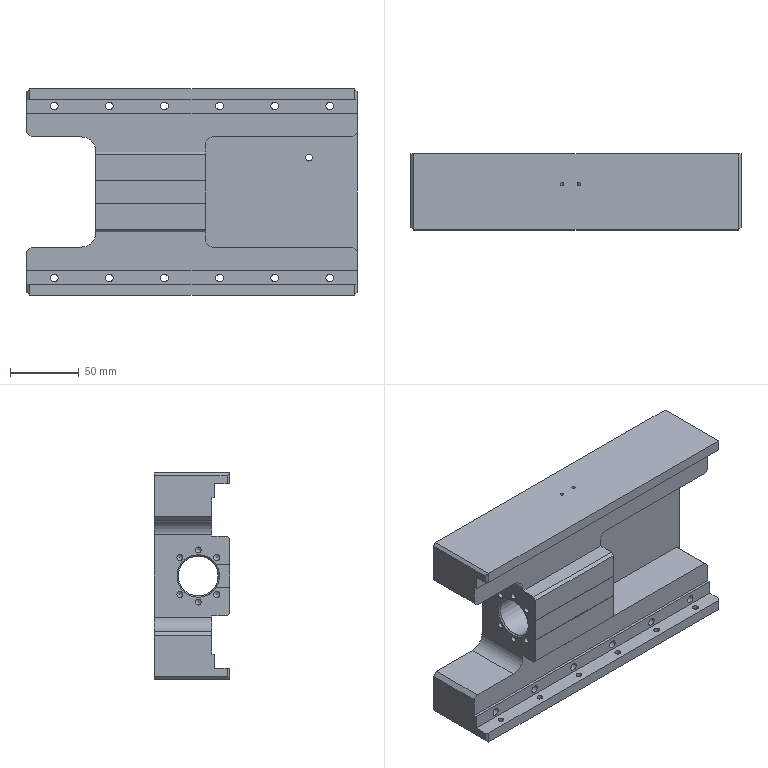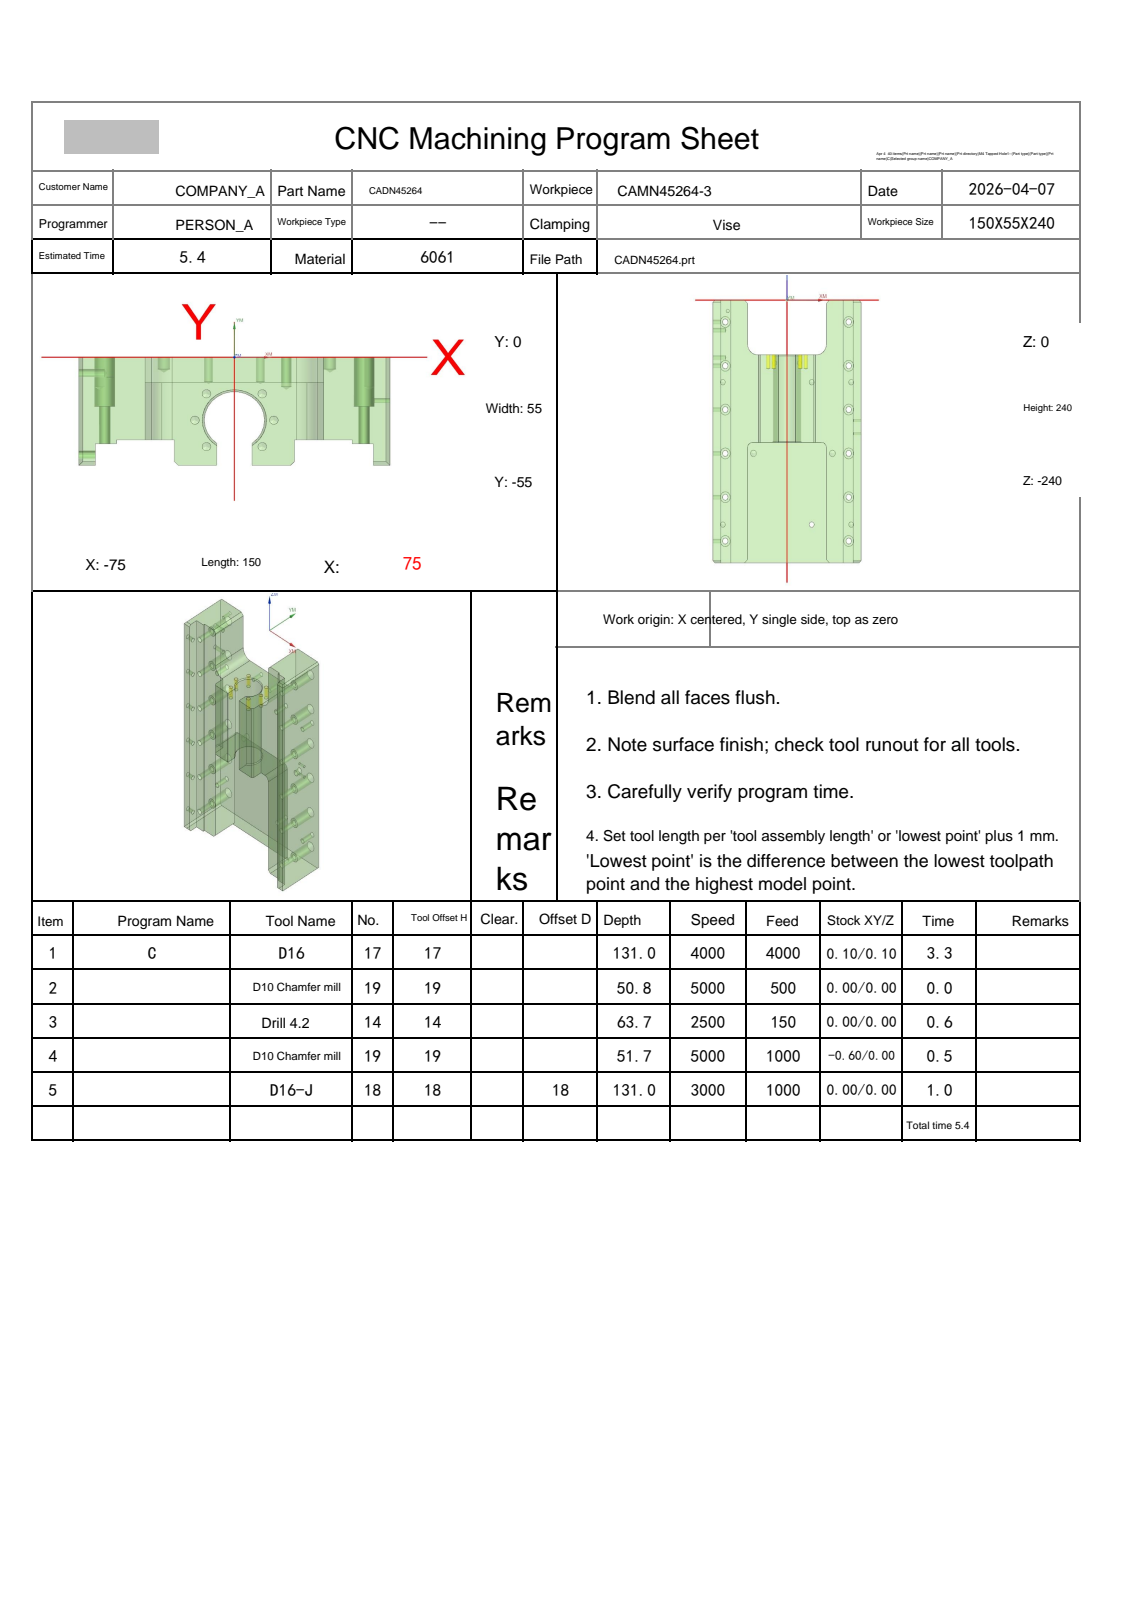NC program | NX | posted by the shop | part box 240 x 55 x 150 mm
Whole program, first 1628 of 1926 lines:
%
O0001
(Machine time: 6.41 MIN)
(===Total Tool:4===)
(T17=D16    D=16.  R=0.   D-  H17 Z=-131. )
(T19=D10 Chamfer mill D=10.  R=0.   D-  H19 Z=-51.7 )
(T14=Drill 4.2  D=4.2  DR_a=118 D-  H14 Z=-63.66)
(T18=D16-J  D=16.  R=0.   D18 H18 Z=-131. )
G80 G90 G17 G49 G40
G91 G28 Z0
M01
N1 T17 M06
(D16  D=16. R=0. H=17 ce=0.10 di=0.10)
G00 G90 G54 X.4 Y-68.796 M03 S4000
G43 H17 Z20.
M08
Z-50.6
G01 Y-54.8 F4000.
Y-44.285
G02 X3.874 Y-37.538 I8.289 J-.001
G03 X6.759 Y-32. I-3.874 J5.538
X0.0 Y-25.241 I-6.759 J0.0
X-6.759 Y-32. I0.0 J-6.759
X-3.908 Y-37.514 I6.759 J0.0
G02 X-.4 Y-44.285 I-4.781 J-6.771
G01 Y-54.8
Y-68.796
G00 Z-51.2
G01 Y-54.8
Y-43.747
G03 X-3.752 Y-37.185 I-8.1 J0.0
G02 X-6.4 Y-32. I3.752 J5.185
X0.0 Y-25.6 I6.4 J0.0
X6.4 Y-32. I0.0 J-6.4
X3.752 Y-37.185 I-6.4 J0.0
G03 X.4 Y-43.747 I4.748 J-6.562
G01 Y-54.8
Y-68.796
G00 Z-51.8
G01 Y-54.8
Y-43.747
G02 X3.752 Y-37.185 I8.1 J0.0
G03 X6.4 Y-32. I-3.752 J5.185
X0.0 Y-25.6 I-6.4 J0.0
X-6.4 Y-32. I0.0 J-6.4
X-3.752 Y-37.185 I6.4 J0.0
G02 X-.4 Y-43.747 I-4.748 J-6.562
G01 Y-54.8
Y-68.796
G00 Z-52.4
G01 Y-54.8
Y-43.747
G03 X-3.752 Y-37.185 I-8.1 J0.0
G02 X-6.4 Y-32. I3.752 J5.185
X0.0 Y-25.6 I6.4 J0.0
X6.4 Y-32. I0.0 J-6.4
X3.752 Y-37.185 I-6.4 J0.0
G03 X.4 Y-43.747 I4.748 J-6.562
G01 Y-54.8
Y-68.796
G00 Z-53.
G01 Y-54.8
Y-43.747
G02 X3.752 Y-37.185 I8.1 J0.0
G03 X6.4 Y-32. I-3.752 J5.185
X0.0 Y-25.6 I-6.4 J0.0
X-6.4 Y-32. I0.0 J-6.4
X-3.752 Y-37.185 I6.4 J0.0
G02 X-.4 Y-43.747 I-4.748 J-6.562
G01 Y-54.8
Y-68.796
G00 Z-53.6
G01 Y-54.8
Y-43.747
G03 X-3.752 Y-37.185 I-8.1 J0.0
G02 X-6.4 Y-32. I3.752 J5.185
X0.0 Y-25.6 I6.4 J0.0
X6.4 Y-32. I0.0 J-6.4
X3.752 Y-37.185 I-6.4 J0.0
G03 X.4 Y-43.747 I4.748 J-6.562
G01 Y-54.8
Y-68.796
G00 Z-54.2
G01 Y-54.8
Y-43.747
G02 X3.752 Y-37.185 I8.1 J0.0
G03 X6.4 Y-32. I-3.752 J5.185
X0.0 Y-25.6 I-6.4 J0.0
X-6.4 Y-32. I0.0 J-6.4
X-3.752 Y-37.185 I6.4 J0.0
G02 X-.4 Y-43.747 I-4.748 J-6.562
G01 Y-54.8
Y-68.796
G00 Z-54.8
G01 Y-54.8
Y-43.747
G03 X-3.752 Y-37.185 I-8.1 J0.0
G02 X-6.4 Y-32. I3.752 J5.185
X0.0 Y-25.6 I6.4 J0.0
X6.4 Y-32. I0.0 J-6.4
X3.752 Y-37.185 I-6.4 J0.0
G03 X.4 Y-43.747 I4.748 J-6.562
G01 Y-54.8
Y-68.796
G00 Z-55.4
G01 Y-54.8
Y-43.747
G02 X3.752 Y-37.185 I8.1 J0.0
G03 X6.4 Y-32. I-3.752 J5.185
X0.0 Y-25.6 I-6.4 J0.0
X-6.4 Y-32. I0.0 J-6.4
X-3.752 Y-37.185 I6.4 J0.0
G02 X-.4 Y-43.747 I-4.748 J-6.562
G01 Y-54.8
Y-68.796
G00 Z-56.
G01 Y-54.8
Y-43.747
G03 X-3.752 Y-37.185 I-8.1 J0.0
G02 X-6.4 Y-32. I3.752 J5.185
X0.0 Y-25.6 I6.4 J0.0
X6.4 Y-32. I0.0 J-6.4
X3.752 Y-37.185 I-6.4 J0.0
G03 X.4 Y-43.747 I4.748 J-6.562
G01 Y-54.8
Y-68.796
G00 Z-56.6
G01 Y-54.8
Y-43.747
G02 X3.752 Y-37.185 I8.1 J0.0
G03 X6.4 Y-32. I-3.752 J5.185
X0.0 Y-25.6 I-6.4 J0.0
X-6.4 Y-32. I0.0 J-6.4
X-3.752 Y-37.185 I6.4 J0.0
G02 X-.4 Y-43.747 I-4.748 J-6.562
G01 Y-54.8
Y-68.796
G00 Z-57.2
G01 Y-54.8
Y-43.747
G03 X-3.752 Y-37.185 I-8.1 J0.0
G02 X-6.4 Y-32. I3.752 J5.185
X0.0 Y-25.6 I6.4 J0.0
X6.4 Y-32. I0.0 J-6.4
X3.752 Y-37.185 I-6.4 J0.0
G03 X.4 Y-43.747 I4.748 J-6.562
G01 Y-54.8
Y-68.796
G00 Z-57.8
G01 Y-54.8
Y-43.747
G02 X3.752 Y-37.185 I8.1 J0.0
G03 X6.4 Y-32. I-3.752 J5.185
X0.0 Y-25.6 I-6.4 J0.0
X-6.4 Y-32. I0.0 J-6.4
X-3.752 Y-37.185 I6.4 J0.0
G02 X-.4 Y-43.747 I-4.748 J-6.562
G01 Y-54.8
Y-68.796
G00 Z-58.4
G01 Y-54.8
Y-43.747
G03 X-3.752 Y-37.185 I-8.1 J0.0
G02 X-6.4 Y-32. I3.752 J5.185
X0.0 Y-25.6 I6.4 J0.0
X6.4 Y-32. I0.0 J-6.4
X3.752 Y-37.185 I-6.4 J0.0
G03 X.4 Y-43.747 I4.748 J-6.562
G01 Y-54.8
Y-68.796
G00 Z-59.
G01 Y-54.8
Y-43.747
G02 X3.752 Y-37.185 I8.1 J0.0
G03 X6.4 Y-32. I-3.752 J5.185
X0.0 Y-25.6 I-6.4 J0.0
X-6.4 Y-32. I0.0 J-6.4
X-3.752 Y-37.185 I6.4 J0.0
G02 X-.4 Y-43.747 I-4.748 J-6.562
G01 Y-54.8
Y-68.796
G00 Z-59.6
G01 Y-54.8
Y-43.747
G03 X-3.752 Y-37.185 I-8.1 J0.0
G02 X-6.4 Y-32. I3.752 J5.185
X0.0 Y-25.6 I6.4 J0.0
X6.4 Y-32. I0.0 J-6.4
X3.752 Y-37.185 I-6.4 J0.0
G03 X.4 Y-43.747 I4.748 J-6.562
G01 Y-54.8
Y-68.796
G00 Z-60.2
G01 Y-54.8
Y-43.747
G02 X3.752 Y-37.185 I8.1 J0.0
G03 X6.4 Y-32. I-3.752 J5.185
X0.0 Y-25.6 I-6.4 J0.0
X-6.4 Y-32. I0.0 J-6.4
X-3.752 Y-37.185 I6.4 J0.0
G02 X-.4 Y-43.747 I-4.748 J-6.562
G01 Y-54.8
Y-68.796
G00 Z-60.8
G01 Y-54.8
Y-43.747
G03 X-3.752 Y-37.185 I-8.1 J0.0
G02 X-6.4 Y-32. I3.752 J5.185
X0.0 Y-25.6 I6.4 J0.0
X6.4 Y-32. I0.0 J-6.4
X3.752 Y-37.185 I-6.4 J0.0
G03 X.4 Y-43.747 I4.748 J-6.562
G01 Y-54.8
Y-68.796
G00 Z-61.4
G01 Y-54.8
Y-43.747
G02 X3.752 Y-37.185 I8.1 J0.0
G03 X6.4 Y-32. I-3.752 J5.185
X0.0 Y-25.6 I-6.4 J0.0
X-6.4 Y-32. I0.0 J-6.4
X-3.752 Y-37.185 I6.4 J0.0
G02 X-.4 Y-43.747 I-4.748 J-6.562
G01 Y-54.8
Y-68.796
G00 Z-62.
G01 Y-54.8
Y-43.747
G03 X-3.752 Y-37.185 I-8.1 J0.0
G02 X-6.4 Y-32. I3.752 J5.185
X0.0 Y-25.6 I6.4 J0.0
X6.4 Y-32. I0.0 J-6.4
X3.752 Y-37.185 I-6.4 J0.0
G03 X.4 Y-43.747 I4.748 J-6.562
G01 Y-54.8
Y-68.796
G00 Z-62.6
G01 Y-54.8
Y-43.747
G02 X3.752 Y-37.185 I8.1 J0.0
G03 X6.4 Y-32. I-3.752 J5.185
X0.0 Y-25.6 I-6.4 J0.0
X-6.4 Y-32. I0.0 J-6.4
X-3.752 Y-37.185 I6.4 J0.0
G02 X-.4 Y-43.747 I-4.748 J-6.562
G01 Y-54.8
Y-68.796
G00 Z-63.2
G01 Y-54.8
Y-43.747
G03 X-3.752 Y-37.185 I-8.1 J0.0
G02 X-6.4 Y-32. I3.752 J5.185
X0.0 Y-25.6 I6.4 J0.0
X6.4 Y-32. I0.0 J-6.4
X3.752 Y-37.185 I-6.4 J0.0
G03 X.4 Y-43.747 I4.748 J-6.562
G01 Y-54.8
Y-68.796
G00 Z-63.8
G01 Y-54.8
Y-43.747
G02 X3.752 Y-37.185 I8.1 J0.0
G03 X6.4 Y-32. I-3.752 J5.185
X0.0 Y-25.6 I-6.4 J0.0
X-6.4 Y-32. I0.0 J-6.4
X-3.752 Y-37.185 I6.4 J0.0
G02 X-.4 Y-43.747 I-4.748 J-6.562
G01 Y-54.8
Y-68.796
G00 Z-64.4
G01 Y-54.8
Y-43.747
G03 X-3.752 Y-37.185 I-8.1 J0.0
G02 X-6.4 Y-32. I3.752 J5.185
X0.0 Y-25.6 I6.4 J0.0
X6.4 Y-32. I0.0 J-6.4
X3.752 Y-37.185 I-6.4 J0.0
G03 X.4 Y-43.747 I4.748 J-6.562
G01 Y-54.8
Y-68.796
G00 Z-65.
G01 Y-54.8
Y-43.747
G02 X3.752 Y-37.185 I8.1 J0.0
G03 X6.4 Y-32. I-3.752 J5.185
X0.0 Y-25.6 I-6.4 J0.0
X-6.4 Y-32. I0.0 J-6.4
X-3.752 Y-37.185 I6.4 J0.0
G02 X-.4 Y-43.747 I-4.748 J-6.562
G01 Y-54.8
Y-68.796
G00 Z-65.6
G01 Y-54.8
Y-43.747
G03 X-3.752 Y-37.185 I-8.1 J0.0
G02 X-6.4 Y-32. I3.752 J5.185
X0.0 Y-25.6 I6.4 J0.0
X6.4 Y-32. I0.0 J-6.4
X3.752 Y-37.185 I-6.4 J0.0
G03 X.4 Y-43.747 I4.748 J-6.562
G01 Y-54.8
Y-68.796
G00 Z-66.2
G01 Y-54.8
Y-43.747
G02 X3.752 Y-37.185 I8.1 J0.0
G03 X6.4 Y-32. I-3.752 J5.185
X0.0 Y-25.6 I-6.4 J0.0
X-6.4 Y-32. I0.0 J-6.4
X-3.752 Y-37.185 I6.4 J0.0
G02 X-.4 Y-43.747 I-4.748 J-6.562
G01 Y-54.8
Y-68.796
G00 Z-66.8
G01 Y-54.8
Y-43.747
G03 X-3.752 Y-37.185 I-8.1 J0.0
G02 X-6.4 Y-32. I3.752 J5.185
X0.0 Y-25.6 I6.4 J0.0
X6.4 Y-32. I0.0 J-6.4
X3.752 Y-37.185 I-6.4 J0.0
G03 X.4 Y-43.747 I4.748 J-6.562
G01 Y-54.8
Y-68.796
G00 Z-67.4
G01 Y-54.8
Y-43.747
G02 X3.752 Y-37.185 I8.1 J0.0
G03 X6.4 Y-32. I-3.752 J5.185
X0.0 Y-25.6 I-6.4 J0.0
X-6.4 Y-32. I0.0 J-6.4
X-3.752 Y-37.185 I6.4 J0.0
G02 X-.4 Y-43.747 I-4.748 J-6.562
G01 Y-54.8
Y-68.796
G00 Z-68.
G01 Y-54.8
Y-43.747
G03 X-3.752 Y-37.185 I-8.1 J0.0
G02 X-6.4 Y-32. I3.752 J5.185
X0.0 Y-25.6 I6.4 J0.0
X6.4 Y-32. I0.0 J-6.4
X3.752 Y-37.185 I-6.4 J0.0
G03 X.4 Y-43.747 I4.748 J-6.562
G01 Y-54.8
Y-68.796
G00 Z-68.6
G01 Y-54.8
Y-43.747
G02 X3.752 Y-37.185 I8.1 J0.0
G03 X6.4 Y-32. I-3.752 J5.185
X0.0 Y-25.6 I-6.4 J0.0
X-6.4 Y-32. I0.0 J-6.4
X-3.752 Y-37.185 I6.4 J0.0
G02 X-.4 Y-43.747 I-4.748 J-6.562
G01 Y-54.8
Y-68.796
G00 Z-69.2
G01 Y-54.8
Y-43.747
G03 X-3.752 Y-37.185 I-8.1 J0.0
G02 X-6.4 Y-32. I3.752 J5.185
X0.0 Y-25.6 I6.4 J0.0
X6.4 Y-32. I0.0 J-6.4
X3.752 Y-37.185 I-6.4 J0.0
G03 X.4 Y-43.747 I4.748 J-6.562
G01 Y-54.8
Y-68.796
G00 Z-69.8
G01 Y-54.8
Y-43.747
G02 X3.752 Y-37.185 I8.1 J0.0
G03 X6.4 Y-32. I-3.752 J5.185
X0.0 Y-25.6 I-6.4 J0.0
X-6.4 Y-32. I0.0 J-6.4
X-3.752 Y-37.185 I6.4 J0.0
G02 X-.4 Y-43.747 I-4.748 J-6.562
G01 Y-54.8
Y-68.796
G00 Z-70.4
G01 Y-54.8
Y-43.747
G03 X-3.752 Y-37.185 I-8.1 J0.0
G02 X-6.4 Y-32. I3.752 J5.185
X0.0 Y-25.6 I6.4 J0.0
X6.4 Y-32. I0.0 J-6.4
X3.752 Y-37.185 I-6.4 J0.0
G03 X.4 Y-43.747 I4.748 J-6.562
G01 Y-54.8
Y-68.796
G00 Z-71.
G01 Y-54.8
Y-43.747
G02 X3.752 Y-37.185 I8.1 J0.0
G03 X6.4 Y-32. I-3.752 J5.185
X0.0 Y-25.6 I-6.4 J0.0
X-6.4 Y-32. I0.0 J-6.4
X-3.752 Y-37.185 I6.4 J0.0
G02 X-.4 Y-43.747 I-4.748 J-6.562
G01 Y-54.8
Y-68.796
G00 Z-71.6
G01 Y-54.8
Y-43.747
G03 X-3.752 Y-37.185 I-8.1 J0.0
G02 X-6.4 Y-32. I3.752 J5.185
X0.0 Y-25.6 I6.4 J0.0
X6.4 Y-32. I0.0 J-6.4
X3.752 Y-37.185 I-6.4 J0.0
G03 X.4 Y-43.747 I4.748 J-6.562
G01 Y-54.8
Y-68.796
G00 Z-72.2
G01 Y-54.8
Y-43.747
G02 X3.752 Y-37.185 I8.1 J0.0
G03 X6.4 Y-32. I-3.752 J5.185
X0.0 Y-25.6 I-6.4 J0.0
X-6.4 Y-32. I0.0 J-6.4
X-3.752 Y-37.185 I6.4 J0.0
G02 X-.4 Y-43.747 I-4.748 J-6.562
G01 Y-54.8
Y-68.796
G00 Z-72.8
G01 Y-54.8
Y-43.747
G03 X-3.752 Y-37.185 I-8.1 J0.0
G02 X-6.4 Y-32. I3.752 J5.185
X0.0 Y-25.6 I6.4 J0.0
X6.4 Y-32. I0.0 J-6.4
X3.752 Y-37.185 I-6.4 J0.0
G03 X.4 Y-43.747 I4.748 J-6.562
G01 Y-54.8
Y-68.796
G00 Z-73.4
G01 Y-54.8
Y-43.747
G02 X3.752 Y-37.185 I8.1 J0.0
G03 X6.4 Y-32. I-3.752 J5.185
X0.0 Y-25.6 I-6.4 J0.0
X-6.4 Y-32. I0.0 J-6.4
X-3.752 Y-37.185 I6.4 J0.0
G02 X-.4 Y-43.747 I-4.748 J-6.562
G01 Y-54.8
Y-68.796
G00 Z-74.
G01 Y-54.8
Y-43.747
G03 X-3.752 Y-37.185 I-8.1 J0.0
G02 X-6.4 Y-32. I3.752 J5.185
X0.0 Y-25.6 I6.4 J0.0
X6.4 Y-32. I0.0 J-6.4
X3.752 Y-37.185 I-6.4 J0.0
G03 X.4 Y-43.747 I4.748 J-6.562
G01 Y-54.8
Y-68.796
G00 Z-74.6
G01 Y-54.8
Y-43.747
G02 X3.752 Y-37.185 I8.1 J0.0
G03 X6.4 Y-32. I-3.752 J5.185
X0.0 Y-25.6 I-6.4 J0.0
X-6.4 Y-32. I0.0 J-6.4
X-3.752 Y-37.185 I6.4 J0.0
G02 X-.4 Y-43.747 I-4.748 J-6.562
G01 Y-54.8
Y-68.796
G00 Z-75.2
G01 Y-54.8
Y-43.747
G03 X-3.752 Y-37.185 I-8.1 J0.0
G02 X-6.4 Y-32. I3.752 J5.185
X0.0 Y-25.6 I6.4 J0.0
X6.4 Y-32. I0.0 J-6.4
X3.752 Y-37.185 I-6.4 J0.0
G03 X.4 Y-43.747 I4.748 J-6.562
G01 Y-54.8
Y-68.796
G00 Z-75.8
G01 Y-54.8
Y-43.747
G02 X3.752 Y-37.185 I8.1 J0.0
G03 X6.4 Y-32. I-3.752 J5.185
X0.0 Y-25.6 I-6.4 J0.0
X-6.4 Y-32. I0.0 J-6.4
X-3.752 Y-37.185 I6.4 J0.0
G02 X-.4 Y-43.747 I-4.748 J-6.562
G01 Y-54.8
Y-68.796
G00 Z-76.4
G01 Y-54.8
Y-43.747
G03 X-3.752 Y-37.185 I-8.1 J0.0
G02 X-6.4 Y-32. I3.752 J5.185
X0.0 Y-25.6 I6.4 J0.0
X6.4 Y-32. I0.0 J-6.4
X3.752 Y-37.185 I-6.4 J0.0
G03 X.4 Y-43.747 I4.748 J-6.562
G01 Y-54.8
Y-68.796
G00 Z-77.
G01 Y-54.8
Y-43.747
G02 X3.752 Y-37.185 I8.1 J0.0
G03 X6.4 Y-32. I-3.752 J5.185
X0.0 Y-25.6 I-6.4 J0.0
X-6.4 Y-32. I0.0 J-6.4
X-3.752 Y-37.185 I6.4 J0.0
G02 X-.4 Y-43.747 I-4.748 J-6.562
G01 Y-54.8
Y-68.796
G00 Z-77.6
G01 Y-54.8
Y-43.747
G03 X-3.752 Y-37.185 I-8.1 J0.0
G02 X-6.4 Y-32. I3.752 J5.185
X0.0 Y-25.6 I6.4 J0.0
X6.4 Y-32. I0.0 J-6.4
X3.752 Y-37.185 I-6.4 J0.0
G03 X.4 Y-43.747 I4.748 J-6.562
G01 Y-54.8
Y-68.796
G00 Z-78.2
G01 Y-54.8
Y-43.747
G02 X3.752 Y-37.185 I8.1 J0.0
G03 X6.4 Y-32. I-3.752 J5.185
X0.0 Y-25.6 I-6.4 J0.0
X-6.4 Y-32. I0.0 J-6.4
X-3.752 Y-37.185 I6.4 J0.0
G02 X-.4 Y-43.747 I-4.748 J-6.562
G01 Y-54.8
Y-68.796
G00 Z-78.8
G01 Y-54.8
Y-43.747
G03 X-3.752 Y-37.185 I-8.1 J0.0
G02 X-6.4 Y-32. I3.752 J5.185
X0.0 Y-25.6 I6.4 J0.0
X6.4 Y-32. I0.0 J-6.4
X3.752 Y-37.185 I-6.4 J0.0
G03 X.4 Y-43.747 I4.748 J-6.562
G01 Y-54.8
Y-68.796
G00 Z-79.4
G01 Y-54.8
Y-43.747
G02 X3.752 Y-37.185 I8.1 J0.0
G03 X6.4 Y-32. I-3.752 J5.185
X0.0 Y-25.6 I-6.4 J0.0
X-6.4 Y-32. I0.0 J-6.4
X-3.752 Y-37.185 I6.4 J0.0
G02 X-.4 Y-43.747 I-4.748 J-6.562
G01 Y-54.8
Y-68.796
G00 Z-80.
G01 Y-54.8
Y-43.747
G03 X-3.752 Y-37.185 I-8.1 J0.0
G02 X-6.4 Y-32. I3.752 J5.185
X0.0 Y-25.6 I6.4 J0.0
X6.4 Y-32. I0.0 J-6.4
X3.752 Y-37.185 I-6.4 J0.0
G03 X.4 Y-43.747 I4.748 J-6.562
G01 Y-54.8
Y-68.796
G00 Z-80.6
G01 Y-54.8
Y-43.747
G02 X3.752 Y-37.185 I8.1 J0.0
G03 X6.4 Y-32. I-3.752 J5.185
X0.0 Y-25.6 I-6.4 J0.0
X-6.4 Y-32. I0.0 J-6.4
X-3.752 Y-37.185 I6.4 J0.0
G02 X-.4 Y-43.747 I-4.748 J-6.562
G01 Y-54.8
Y-68.796
G00 Z-81.2
G01 Y-54.8
Y-43.747
G03 X-3.752 Y-37.185 I-8.1 J0.0
G02 X-6.4 Y-32. I3.752 J5.185
X0.0 Y-25.6 I6.4 J0.0
X6.4 Y-32. I0.0 J-6.4
X3.752 Y-37.185 I-6.4 J0.0
G03 X.4 Y-43.747 I4.748 J-6.562
G01 Y-54.8
Y-68.796
G00 Z-81.8
G01 Y-54.8
Y-43.747
G02 X3.752 Y-37.185 I8.1 J0.0
G03 X6.4 Y-32. I-3.752 J5.185
X0.0 Y-25.6 I-6.4 J0.0
X-6.4 Y-32. I0.0 J-6.4
X-3.752 Y-37.185 I6.4 J0.0
G02 X-.4 Y-43.747 I-4.748 J-6.562
G01 Y-54.8
Y-68.796
G00 Z-82.4
G01 Y-54.8
Y-43.747
G03 X-3.752 Y-37.185 I-8.1 J0.0
G02 X-6.4 Y-32. I3.752 J5.185
X0.0 Y-25.6 I6.4 J0.0
X6.4 Y-32. I0.0 J-6.4
X3.752 Y-37.185 I-6.4 J0.0
G03 X.4 Y-43.747 I4.748 J-6.562
G01 Y-54.8
Y-68.796
G00 Z-83.
G01 Y-54.8
Y-43.747
G02 X3.752 Y-37.185 I8.1 J0.0
G03 X6.4 Y-32. I-3.752 J5.185
X0.0 Y-25.6 I-6.4 J0.0
X-6.4 Y-32. I0.0 J-6.4
X-3.752 Y-37.185 I6.4 J0.0
G02 X-.4 Y-43.747 I-4.748 J-6.562
G01 Y-54.8
Y-68.796
G00 Z-83.6
G01 Y-54.8
Y-43.747
G03 X-3.752 Y-37.185 I-8.1 J0.0
G02 X-6.4 Y-32. I3.752 J5.185
X0.0 Y-25.6 I6.4 J0.0
X6.4 Y-32. I0.0 J-6.4
X3.752 Y-37.185 I-6.4 J0.0
G03 X.4 Y-43.747 I4.748 J-6.562
G01 Y-54.8
Y-68.796
G00 Z-84.2
G01 Y-54.8
Y-43.747
G02 X3.752 Y-37.185 I8.1 J0.0
G03 X6.4 Y-32. I-3.752 J5.185
X0.0 Y-25.6 I-6.4 J0.0
X-6.4 Y-32. I0.0 J-6.4
X-3.752 Y-37.185 I6.4 J0.0
G02 X-.4 Y-43.747 I-4.748 J-6.562
G01 Y-54.8
Y-68.796
G00 Z-84.8
G01 Y-54.8
Y-43.747
G03 X-3.752 Y-37.185 I-8.1 J0.0
G02 X-6.4 Y-32. I3.752 J5.185
X0.0 Y-25.6 I6.4 J0.0
X6.4 Y-32. I0.0 J-6.4
X3.752 Y-37.185 I-6.4 J0.0
G03 X.4 Y-43.747 I4.748 J-6.562
G01 Y-54.8
Y-68.796
G00 Z-85.4
G01 Y-54.8
Y-43.747
G02 X3.752 Y-37.185 I8.1 J0.0
G03 X6.4 Y-32. I-3.752 J5.185
X0.0 Y-25.6 I-6.4 J0.0
X-6.4 Y-32. I0.0 J-6.4
X-3.752 Y-37.185 I6.4 J0.0
G02 X-.4 Y-43.747 I-4.748 J-6.562
G01 Y-54.8
Y-68.796
G00 Z-86.
G01 Y-54.8
Y-43.747
G03 X-3.752 Y-37.185 I-8.1 J0.0
G02 X-6.4 Y-32. I3.752 J5.185
X0.0 Y-25.6 I6.4 J0.0
X6.4 Y-32. I0.0 J-6.4
X3.752 Y-37.185 I-6.4 J0.0
G03 X.4 Y-43.747 I4.748 J-6.562
G01 Y-54.8
Y-68.796
G00 Z-86.6
G01 Y-54.8
Y-43.747
G02 X3.752 Y-37.185 I8.1 J0.0
G03 X6.4 Y-32. I-3.752 J5.185
X0.0 Y-25.6 I-6.4 J0.0
X-6.4 Y-32. I0.0 J-6.4
X-3.752 Y-37.185 I6.4 J0.0
G02 X-.4 Y-43.747 I-4.748 J-6.562
G01 Y-54.8
Y-68.796
G00 Z-87.2
G01 Y-54.8
Y-43.747
G03 X-3.752 Y-37.185 I-8.1 J0.0
G02 X-6.4 Y-32. I3.752 J5.185
X0.0 Y-25.6 I6.4 J0.0
X6.4 Y-32. I0.0 J-6.4
X3.752 Y-37.185 I-6.4 J0.0
G03 X.4 Y-43.747 I4.748 J-6.562
G01 Y-54.8
Y-68.796
G00 Z-87.8
G01 Y-54.8
Y-43.747
G02 X3.752 Y-37.185 I8.1 J0.0
G03 X6.4 Y-32. I-3.752 J5.185
X0.0 Y-25.6 I-6.4 J0.0
X-6.4 Y-32. I0.0 J-6.4
X-3.752 Y-37.185 I6.4 J0.0
G02 X-.4 Y-43.747 I-4.748 J-6.562
G01 Y-54.8
Y-68.796
G00 Z-88.4
G01 Y-54.8
Y-43.747
G03 X-3.752 Y-37.185 I-8.1 J0.0
G02 X-6.4 Y-32. I3.752 J5.185
X0.0 Y-25.6 I6.4 J0.0
X6.4 Y-32. I0.0 J-6.4
X3.752 Y-37.185 I-6.4 J0.0
G03 X.4 Y-43.747 I4.748 J-6.562
G01 Y-54.8
Y-68.796
G00 Z-89.
G01 Y-54.8
Y-43.747
G02 X3.752 Y-37.185 I8.1 J0.0
G03 X6.4 Y-32. I-3.752 J5.185
X0.0 Y-25.6 I-6.4 J0.0
X-6.4 Y-32. I0.0 J-6.4
X-3.752 Y-37.185 I6.4 J0.0
G02 X-.4 Y-43.747 I-4.748 J-6.562
G01 Y-54.8
Y-68.796
G00 Z-89.6
G01 Y-54.8
Y-43.747
G03 X-3.752 Y-37.185 I-8.1 J0.0
G02 X-6.4 Y-32. I3.752 J5.185
X0.0 Y-25.6 I6.4 J0.0
X6.4 Y-32. I0.0 J-6.4
X3.752 Y-37.185 I-6.4 J0.0
G03 X.4 Y-43.747 I4.748 J-6.562
G01 Y-54.8
Y-68.796
G00 Z-90.2
G01 Y-54.8
Y-43.747
G02 X3.752 Y-37.185 I8.1 J0.0
G03 X6.4 Y-32. I-3.752 J5.185
X0.0 Y-25.6 I-6.4 J0.0
X-6.4 Y-32. I0.0 J-6.4
X-3.752 Y-37.185 I6.4 J0.0
G02 X-.4 Y-43.747 I-4.748 J-6.562
G01 Y-54.8
Y-68.796
G00 Z-90.8
G01 Y-54.8
Y-43.747
G03 X-3.752 Y-37.185 I-8.1 J0.0
G02 X-6.4 Y-32. I3.752 J5.185
X0.0 Y-25.6 I6.4 J0.0
X6.4 Y-32. I0.0 J-6.4
X3.752 Y-37.185 I-6.4 J0.0
G03 X.4 Y-43.747 I4.748 J-6.562
G01 Y-54.8
Y-68.796
G00 Z-91.4
G01 Y-54.8
Y-43.747
G02 X3.752 Y-37.185 I8.1 J0.0
G03 X6.4 Y-32. I-3.752 J5.185
X0.0 Y-25.6 I-6.4 J0.0
X-6.4 Y-32. I0.0 J-6.4
X-3.752 Y-37.185 I6.4 J0.0
G02 X-.4 Y-43.747 I-4.748 J-6.562
G01 Y-54.8
Y-68.796
G00 Z-92.
G01 Y-54.8
Y-43.747
G03 X-3.752 Y-37.185 I-8.1 J0.0
G02 X-6.4 Y-32. I3.752 J5.185
X0.0 Y-25.6 I6.4 J0.0
X6.4 Y-32. I0.0 J-6.4
X3.752 Y-37.185 I-6.4 J0.0
G03 X.4 Y-43.747 I4.748 J-6.562
G01 Y-54.8
Y-68.796
G00 Z-92.6
G01 Y-54.8
Y-43.747
G02 X3.752 Y-37.185 I8.1 J0.0
G03 X6.4 Y-32. I-3.752 J5.185
X0.0 Y-25.6 I-6.4 J0.0
X-6.4 Y-32. I0.0 J-6.4
X-3.752 Y-37.185 I6.4 J0.0
G02 X-.4 Y-43.747 I-4.748 J-6.562
G01 Y-54.8
Y-68.796
G00 Z-93.2
G01 Y-54.8
Y-43.747
G03 X-3.752 Y-37.185 I-8.1 J0.0
G02 X-6.4 Y-32. I3.752 J5.185
X0.0 Y-25.6 I6.4 J0.0
X6.4 Y-32. I0.0 J-6.4
X3.752 Y-37.185 I-6.4 J0.0
G03 X.4 Y-43.747 I4.748 J-6.562
G01 Y-54.8
Y-68.796
G00 Z-93.8
G01 Y-54.8
Y-43.747
G02 X3.752 Y-37.185 I8.1 J0.0
G03 X6.4 Y-32. I-3.752 J5.185
X0.0 Y-25.6 I-6.4 J0.0
X-6.4 Y-32. I0.0 J-6.4
X-3.752 Y-37.185 I6.4 J0.0
G02 X-.4 Y-43.747 I-4.748 J-6.562
G01 Y-54.8
Y-68.796
G00 Z-94.4
G01 Y-54.8
Y-43.747
G03 X-3.752 Y-37.185 I-8.1 J0.0
G02 X-6.4 Y-32. I3.752 J5.185
X0.0 Y-25.6 I6.4 J0.0
X6.4 Y-32. I0.0 J-6.4
X3.752 Y-37.185 I-6.4 J0.0
G03 X.4 Y-43.747 I4.748 J-6.562
G01 Y-54.8
Y-68.796
G00 Z-95.
G01 Y-54.8
Y-43.747
G02 X3.752 Y-37.185 I8.1 J0.0
G03 X6.4 Y-32. I-3.752 J5.185
X0.0 Y-25.6 I-6.4 J0.0
X-6.4 Y-32. I0.0 J-6.4
X-3.752 Y-37.185 I6.4 J0.0
G02 X-.4 Y-43.747 I-4.748 J-6.562
G01 Y-54.8
Y-68.796
G00 Z-95.6
G01 Y-54.8
Y-43.747
G03 X-3.752 Y-37.185 I-8.1 J0.0
G02 X-6.4 Y-32. I3.752 J5.185
X0.0 Y-25.6 I6.4 J0.0
X6.4 Y-32. I0.0 J-6.4
X3.752 Y-37.185 I-6.4 J0.0
G03 X.4 Y-43.747 I4.748 J-6.562
G01 Y-54.8
Y-68.796
G00 Z-96.2
G01 Y-54.8
Y-43.747
G02 X3.752 Y-37.185 I8.1 J0.0
G03 X6.4 Y-32. I-3.752 J5.185
X0.0 Y-25.6 I-6.4 J0.0
X-6.4 Y-32. I0.0 J-6.4
X-3.752 Y-37.185 I6.4 J0.0
G02 X-.4 Y-43.747 I-4.748 J-6.562
G01 Y-54.8
Y-68.796
G00 Z-96.8
G01 Y-54.8
Y-43.747
G03 X-3.752 Y-37.185 I-8.1 J0.0
G02 X-6.4 Y-32. I3.752 J5.185
X0.0 Y-25.6 I6.4 J0.0
X6.4 Y-32. I0.0 J-6.4
X3.752 Y-37.185 I-6.4 J0.0
G03 X.4 Y-43.747 I4.748 J-6.562
G01 Y-54.8
Y-68.796
G00 Z-97.4
G01 Y-54.8
Y-43.747
G02 X3.752 Y-37.185 I8.1 J0.0
G03 X6.4 Y-32. I-3.752 J5.185
X0.0 Y-25.6 I-6.4 J0.0
X-6.4 Y-32. I0.0 J-6.4
X-3.752 Y-37.185 I6.4 J0.0
G02 X-.4 Y-43.747 I-4.748 J-6.562
G01 Y-54.8
Y-68.796
G00 Z-98.
G01 Y-54.8
Y-43.747
G03 X-3.752 Y-37.185 I-8.1 J0.0
G02 X-6.4 Y-32. I3.752 J5.185
X0.0 Y-25.6 I6.4 J0.0
X6.4 Y-32. I0.0 J-6.4
X3.752 Y-37.185 I-6.4 J0.0
G03 X.4 Y-43.747 I4.748 J-6.562
G01 Y-54.8
Y-68.796
G00 Z-98.6
G01 Y-54.8
Y-43.747
G02 X3.752 Y-37.185 I8.1 J0.0
G03 X6.4 Y-32. I-3.752 J5.185
X0.0 Y-25.6 I-6.4 J0.0
X-6.4 Y-32. I0.0 J-6.4
X-3.752 Y-37.185 I6.4 J0.0
G02 X-.4 Y-43.747 I-4.748 J-6.562
G01 Y-54.8
Y-68.796
G00 Z-99.2
G01 Y-54.8
Y-43.747
G03 X-3.752 Y-37.185 I-8.1 J0.0
G02 X-6.4 Y-32. I3.752 J5.185
X0.0 Y-25.6 I6.4 J0.0
X6.4 Y-32. I0.0 J-6.4
X3.752 Y-37.185 I-6.4 J0.0
G03 X.4 Y-43.747 I4.748 J-6.562
G01 Y-54.8
Y-68.796
G00 Z-99.8
G01 Y-54.8
Y-43.747
G02 X3.752 Y-37.185 I8.1 J0.0
G03 X6.4 Y-32. I-3.752 J5.185
X0.0 Y-25.6 I-6.4 J0.0
X-6.4 Y-32. I0.0 J-6.4
X-3.752 Y-37.185 I6.4 J0.0
G02 X-.4 Y-43.747 I-4.748 J-6.562
G01 Y-54.8
Y-68.796
G00 Z-100.4
G01 Y-54.8
Y-43.747
G03 X-3.752 Y-37.185 I-8.1 J0.0
G02 X-6.4 Y-32. I3.752 J5.185
X0.0 Y-25.6 I6.4 J0.0
X6.4 Y-32. I0.0 J-6.4
X3.752 Y-37.185 I-6.4 J0.0
G03 X.4 Y-43.747 I4.748 J-6.562
G01 Y-54.8
Y-68.796
G00 Z-101.
G01 Y-54.8
Y-43.747
G02 X3.752 Y-37.185 I8.1 J0.0
G03 X6.4 Y-32. I-3.752 J5.185
X0.0 Y-25.6 I-6.4 J0.0
X-6.4 Y-32. I0.0 J-6.4
X-3.752 Y-37.185 I6.4 J0.0
G02 X-.4 Y-43.747 I-4.748 J-6.562
G01 Y-54.8
Y-68.796
G00 Z-101.6
G01 Y-54.8
Y-43.747
G03 X-3.752 Y-37.185 I-8.1 J0.0
G02 X-6.4 Y-32. I3.752 J5.185
X0.0 Y-25.6 I6.4 J0.0
X6.4 Y-32. I0.0 J-6.4
X3.752 Y-37.185 I-6.4 J0.0
G03 X.4 Y-43.747 I4.748 J-6.562
G01 Y-54.8
Y-68.796
G00 Z-102.2
G01 Y-54.8
Y-43.747
G02 X3.752 Y-37.185 I8.1 J0.0
G03 X6.4 Y-32. I-3.752 J5.185
X0.0 Y-25.6 I-6.4 J0.0
X-6.4 Y-32. I0.0 J-6.4
X-3.752 Y-37.185 I6.4 J0.0
G02 X-.4 Y-43.747 I-4.748 J-6.562
G01 Y-54.8
Y-68.796
G00 Z-102.8
G01 Y-54.8
Y-43.747
G03 X-3.752 Y-37.185 I-8.1 J0.0
G02 X-6.4 Y-32. I3.752 J5.185
X0.0 Y-25.6 I6.4 J0.0
X6.4 Y-32. I0.0 J-6.4
X3.752 Y-37.185 I-6.4 J0.0
G03 X.4 Y-43.747 I4.748 J-6.562
G01 Y-54.8
Y-68.796
G00 Z-103.4
G01 Y-54.8
Y-43.747
G02 X3.752 Y-37.185 I8.1 J0.0
G03 X6.4 Y-32. I-3.752 J5.185
X0.0 Y-25.6 I-6.4 J0.0
X-6.4 Y-32. I0.0 J-6.4
X-3.752 Y-37.185 I6.4 J0.0
G02 X-.4 Y-43.747 I-4.748 J-6.562
G01 Y-54.8
Y-68.796
G00 Z-104.
G01 Y-54.8
Y-43.747
G03 X-3.752 Y-37.185 I-8.1 J0.0
G02 X-6.4 Y-32. I3.752 J5.185
X0.0 Y-25.6 I6.4 J0.0
X6.4 Y-32. I0.0 J-6.4
X3.752 Y-37.185 I-6.4 J0.0
G03 X.4 Y-43.747 I4.748 J-6.562
G01 Y-54.8
Y-68.796
G00 Z-104.6
G01 Y-54.8
Y-43.747
G02 X3.752 Y-37.185 I8.1 J0.0
G03 X6.4 Y-32. I-3.752 J5.185
X0.0 Y-25.6 I-6.4 J0.0
X-6.4 Y-32. I0.0 J-6.4
X-3.752 Y-37.185 I6.4 J0.0
G02 X-.4 Y-43.747 I-4.748 J-6.562
G01 Y-54.8
Y-68.796
G00 Z-105.2
G01 Y-54.8
Y-43.747
G03 X-3.752 Y-37.185 I-8.1 J0.0
G02 X-6.4 Y-32. I3.752 J5.185
X0.0 Y-25.6 I6.4 J0.0
X6.4 Y-32. I0.0 J-6.4
X3.752 Y-37.185 I-6.4 J0.0
G03 X.4 Y-43.747 I4.748 J-6.562
G01 Y-54.8
Y-68.796
G00 Z-105.8
G01 Y-54.8
Y-43.747
G02 X3.752 Y-37.185 I8.1 J0.0
G03 X6.4 Y-32. I-3.752 J5.185
X0.0 Y-25.6 I-6.4 J0.0
X-6.4 Y-32. I0.0 J-6.4
X-3.752 Y-37.185 I6.4 J0.0
G02 X-.4 Y-43.747 I-4.748 J-6.562
G01 Y-54.8
Y-68.796
G00 Z-106.4
G01 Y-54.8
Y-43.747
G03 X-3.752 Y-37.185 I-8.1 J0.0
G02 X-6.4 Y-32. I3.752 J5.185
X0.0 Y-25.6 I6.4 J0.0
X6.4 Y-32. I0.0 J-6.4
X3.752 Y-37.185 I-6.4 J0.0
G03 X.4 Y-43.747 I4.748 J-6.562
G01 Y-54.8
Y-68.796
G00 Z-107.
G01 Y-54.8
Y-43.747
G02 X3.752 Y-37.185 I8.1 J0.0
G03 X6.4 Y-32. I-3.752 J5.185
X0.0 Y-25.6 I-6.4 J0.0
X-6.4 Y-32. I0.0 J-6.4
X-3.752 Y-37.185 I6.4 J0.0
G02 X-.4 Y-43.747 I-4.748 J-6.562
G01 Y-54.8
Y-68.796
G00 Z-107.6
G01 Y-54.8
Y-43.747
G03 X-3.752 Y-37.185 I-8.1 J0.0
G02 X-6.4 Y-32. I3.752 J5.185
X0.0 Y-25.6 I6.4 J0.0
X6.4 Y-32. I0.0 J-6.4
X3.752 Y-37.185 I-6.4 J0.0
G03 X.4 Y-43.747 I4.748 J-6.562
G01 Y-54.8
Y-68.796
G00 Z-108.2
G01 Y-54.8
Y-43.747
G02 X3.752 Y-37.185 I8.1 J0.0
G03 X6.4 Y-32. I-3.752 J5.185
X0.0 Y-25.6 I-6.4 J0.0
X-6.4 Y-32. I0.0 J-6.4
X-3.752 Y-37.185 I6.4 J0.0
G02 X-.4 Y-43.747 I-4.748 J-6.562
G01 Y-54.8
Y-68.796
G00 Z-108.8
G01 Y-54.8
Y-43.747
G03 X-3.752 Y-37.185 I-8.1 J0.0
G02 X-6.4 Y-32. I3.752 J5.185
X0.0 Y-25.6 I6.4 J0.0
X6.4 Y-32. I0.0 J-6.4
X3.752 Y-37.185 I-6.4 J0.0
G03 X.4 Y-43.747 I4.748 J-6.562
G01 Y-54.8
Y-68.796
G00 Z-109.4
G01 Y-54.8
Y-43.747
G02 X3.752 Y-37.185 I8.1 J0.0
G03 X6.4 Y-32. I-3.752 J5.185
X0.0 Y-25.6 I-6.4 J0.0
X-6.4 Y-32. I0.0 J-6.4
X-3.752 Y-37.185 I6.4 J0.0
G02 X-.4 Y-43.747 I-4.748 J-6.562
G01 Y-54.8
Y-68.796
G00 Z-110.
G01 Y-54.8
Y-43.747
G03 X-3.752 Y-37.185 I-8.1 J0.0
G02 X-6.4 Y-32. I3.752 J5.185
X0.0 Y-25.6 I6.4 J0.0
X6.4 Y-32. I0.0 J-6.4
X3.752 Y-37.185 I-6.4 J0.0
G03 X.4 Y-43.747 I4.748 J-6.562
G01 Y-54.8
Y-68.796
G00 Z-110.6
G01 Y-54.8
Y-43.747
G02 X3.752 Y-37.185 I8.1 J0.0
G03 X6.4 Y-32. I-3.752 J5.185
X0.0 Y-25.6 I-6.4 J0.0
X-6.4 Y-32. I0.0 J-6.4
X-3.752 Y-37.185 I6.4 J0.0
G02 X-.4 Y-43.747 I-4.748 J-6.562
G01 Y-54.8
Y-68.796
G00 Z-111.2
G01 Y-54.8
Y-43.747
G03 X-3.752 Y-37.185 I-8.1 J0.0
G02 X-6.4 Y-32. I3.752 J5.185
X0.0 Y-25.6 I6.4 J0.0
X6.4 Y-32. I0.0 J-6.4
X3.752 Y-37.185 I-6.4 J0.0
G03 X.4 Y-43.747 I4.748 J-6.562
G01 Y-54.8
Y-68.796
G00 Z-111.8
G01 Y-54.8
Y-43.747
G02 X3.752 Y-37.185 I8.1 J0.0
G03 X6.4 Y-32. I-3.752 J5.185
X0.0 Y-25.6 I-6.4 J0.0
X-6.4 Y-32. I0.0 J-6.4
X-3.752 Y-37.185 I6.4 J0.0
G02 X-.4 Y-43.747 I-4.748 J-6.562
G01 Y-54.8
Y-68.796
G00 Z-112.4
G01 Y-54.8
Y-43.747
G03 X-3.752 Y-37.185 I-8.1 J0.0
G02 X-6.4 Y-32. I3.752 J5.185
X0.0 Y-25.6 I6.4 J0.0
X6.4 Y-32. I0.0 J-6.4
X3.752 Y-37.185 I-6.4 J0.0
G03 X.4 Y-43.747 I4.748 J-6.562
G01 Y-54.8
Y-68.796
G00 Z-113.
G01 Y-54.8
Y-43.747
G02 X3.752 Y-37.185 I8.1 J0.0
G03 X6.4 Y-32. I-3.752 J5.185
X0.0 Y-25.6 I-6.4 J0.0
X-6.4 Y-32. I0.0 J-6.4
X-3.752 Y-37.185 I6.4 J0.0
G02 X-.4 Y-43.747 I-4.748 J-6.562
G01 Y-54.8
Y-68.796
G00 Z-113.6
G01 Y-54.8
Y-43.747
G03 X-3.752 Y-37.185 I-8.1 J0.0
G02 X-6.4 Y-32. I3.752 J5.185
X0.0 Y-25.6 I6.4 J0.0
X6.4 Y-32. I0.0 J-6.4
X3.752 Y-37.185 I-6.4 J0.0
G03 X.4 Y-43.747 I4.748 J-6.562
G01 Y-54.8
Y-68.796
G00 Z-114.2
G01 Y-54.8
Y-43.747
G02 X3.752 Y-37.185 I8.1 J0.0
G03 X6.4 Y-32. I-3.752 J5.185
X0.0 Y-25.6 I-6.4 J0.0
X-6.4 Y-32. I0.0 J-6.4
X-3.752 Y-37.185 I6.4 J0.0
G02 X-.4 Y-43.747 I-4.748 J-6.562
G01 Y-54.8
Y-68.796
G00 Z-114.8
G01 Y-54.8
Y-43.747
G03 X-3.752 Y-37.185 I-8.1 J0.0
G02 X-6.4 Y-32. I3.752 J5.185
X0.0 Y-25.6 I6.4 J0.0
X6.4 Y-32. I0.0 J-6.4
X3.752 Y-37.185 I-6.4 J0.0
G03 X.4 Y-43.747 I4.748 J-6.562
G01 Y-54.8
Y-68.796
G00 Z-115.4
G01 Y-54.8
Y-43.747
G02 X3.752 Y-37.185 I8.1 J0.0
G03 X6.4 Y-32. I-3.752 J5.185
X0.0 Y-25.6 I-6.4 J0.0
X-6.4 Y-32. I0.0 J-6.4
X-3.752 Y-37.185 I6.4 J0.0
G02 X-.4 Y-43.747 I-4.748 J-6.562
G01 Y-54.8
Y-68.796
G00 Z-116.
G01 Y-54.8
Y-43.747
G03 X-3.752 Y-37.185 I-8.1 J0.0
G02 X-6.4 Y-32. I3.752 J5.185
X0.0 Y-25.6 I6.4 J0.0
X6.4 Y-32. I0.0 J-6.4
X3.752 Y-37.185 I-6.4 J0.0
G03 X.4 Y-43.747 I4.748 J-6.562
G01 Y-54.8
Y-68.796
G00 Z-116.6
G01 Y-54.8
Y-43.747
G02 X3.752 Y-37.185 I8.1 J0.0
G03 X6.4 Y-32. I-3.752 J5.185
X0.0 Y-25.6 I-6.4 J0.0
X-6.4 Y-32. I0.0 J-6.4
X-3.752 Y-37.185 I6.4 J0.0
G02 X-.4 Y-43.747 I-4.748 J-6.562
G01 Y-54.8
Y-68.796
G00 Z-117.2
G01 Y-54.8
Y-43.747
G03 X-3.752 Y-37.185 I-8.1 J0.0
G02 X-6.4 Y-32. I3.752 J5.185
X0.0 Y-25.6 I6.4 J0.0
X6.4 Y-32. I0.0 J-6.4
X3.752 Y-37.185 I-6.4 J0.0
G03 X.4 Y-43.747 I4.748 J-6.562
G01 Y-54.8
Y-68.796
G00 Z-117.8
G01 Y-54.8
Y-43.747
G02 X3.752 Y-37.185 I8.1 J0.0
G03 X6.4 Y-32. I-3.752 J5.185
X0.0 Y-25.6 I-6.4 J0.0
X-6.4 Y-32. I0.0 J-6.4
X-3.752 Y-37.185 I6.4 J0.0
G02 X-.4 Y-43.747 I-4.748 J-6.562
G01 Y-54.8
Y-68.796
G00 Z-118.4
G01 Y-54.8
Y-43.747
G03 X-3.752 Y-37.185 I-8.1 J0.0
G02 X-6.4 Y-32. I3.752 J5.185
X0.0 Y-25.6 I6.4 J0.0
X6.4 Y-32. I0.0 J-6.4
X3.752 Y-37.185 I-6.4 J0.0
G03 X.4 Y-43.747 I4.748 J-6.562
G01 Y-54.8
Y-68.796
G00 Z-119.
G01 Y-54.8
Y-43.747
G02 X3.752 Y-37.185 I8.1 J0.0
G03 X6.4 Y-32. I-3.752 J5.185
X0.0 Y-25.6 I-6.4 J0.0
X-6.4 Y-32. I0.0 J-6.4
X-3.752 Y-37.185 I6.4 J0.0
G02 X-.4 Y-43.747 I-4.748 J-6.562
G01 Y-54.8
Y-68.796
G00 Z-119.6
G01 Y-54.8
Y-43.747
G03 X-3.752 Y-37.185 I-8.1 J0.0
G02 X-6.4 Y-32. I3.752 J5.185
X0.0 Y-25.6 I6.4 J0.0
X6.4 Y-32. I0.0 J-6.4
X3.752 Y-37.185 I-6.4 J0.0
G03 X.4 Y-43.747 I4.748 J-6.562
G01 Y-54.8
Y-68.796
G00 Z-120.2
G01 Y-54.8
Y-43.747
G02 X3.752 Y-37.185 I8.1 J0.0
G03 X6.4 Y-32. I-3.752 J5.185
X0.0 Y-25.6 I-6.4 J0.0
X-6.4 Y-32. I0.0 J-6.4
X-3.752 Y-37.185 I6.4 J0.0
G02 X-.4 Y-43.747 I-4.748 J-6.562
G01 Y-54.8
Y-68.796
G00 Z-120.8
G01 Y-54.8
Y-43.747
G03 X-3.752 Y-37.185 I-8.1 J0.0
G02 X-6.4 Y-32. I3.752 J5.185
X0.0 Y-25.6 I6.4 J0.0
X6.4 Y-32. I0.0 J-6.4
X3.752 Y-37.185 I-6.4 J0.0
G03 X.4 Y-43.747 I4.748 J-6.562
G01 Y-54.8
Y-68.796
G00 Z-121.4
G01 Y-54.8
Y-43.747
G02 X3.752 Y-37.185 I8.1 J0.0
G03 X6.4 Y-32. I-3.752 J5.185
X0.0 Y-25.6 I-6.4 J0.0
X-6.4 Y-32. I0.0 J-6.4
X-3.752 Y-37.185 I6.4 J0.0
G02 X-.4 Y-43.747 I-4.748 J-6.562
G01 Y-54.8
Y-68.796
G00 Z-122.
G01 Y-54.8
Y-43.747
G03 X-3.752 Y-37.185 I-8.1 J0.0
G02 X-6.4 Y-32. I3.752 J5.185
X0.0 Y-25.6 I6.4 J0.0
X6.4 Y-32. I0.0 J-6.4
X3.752 Y-37.185 I-6.4 J0.0
G03 X.4 Y-43.747 I4.748 J-6.562
G01 Y-54.8
Y-68.796
G00 Z-122.6
G01 Y-54.8
Y-43.747
G02 X3.752 Y-37.185 I8.1 J0.0
G03 X6.4 Y-32. I-3.752 J5.185
X0.0 Y-25.6 I-6.4 J0.0
X-6.4 Y-32. I0.0 J-6.4
X-3.752 Y-37.185 I6.4 J0.0
G02 X-.4 Y-43.747 I-4.748 J-6.562
G01 Y-54.8
Y-68.796
G00 Z-123.2
G01 Y-54.8
Y-43.747
G03 X-3.752 Y-37.185 I-8.1 J0.0
G02 X-6.4 Y-32. I3.752 J5.185
X0.0 Y-25.6 I6.4 J0.0
X6.4 Y-32. I0.0 J-6.4
X3.752 Y-37.185 I-6.4 J0.0
G03 X.4 Y-43.747 I4.748 J-6.562
G01 Y-54.8
Y-68.796
G00 Z-123.8
G01 Y-54.8
Y-43.747
G02 X3.752 Y-37.185 I8.1 J0.0
G03 X6.4 Y-32. I-3.752 J5.185
X0.0 Y-25.6 I-6.4 J0.0
X-6.4 Y-32. I0.0 J-6.4
X-3.752 Y-37.185 I6.4 J0.0
G02 X-.4 Y-43.747 I-4.748 J-6.562
G01 Y-54.8
Y-68.796
G00 Z-124.4
G01 Y-54.8
Y-43.747
G03 X-3.752 Y-37.185 I-8.1 J0.0
G02 X-6.4 Y-32. I3.752 J5.185
X0.0 Y-25.6 I6.4 J0.0
X6.4 Y-32. I0.0 J-6.4
X3.752 Y-37.185 I-6.4 J0.0
G03 X.4 Y-43.747 I4.748 J-6.562
G01 Y-54.8
Y-68.796
G00 Z-125.
G01 Y-54.8
Y-43.747
G02 X3.752 Y-37.185 I8.1 J0.0
G03 X6.4 Y-32. I-3.752 J5.185
X0.0 Y-25.6 I-6.4 J0.0
X-6.4 Y-32. I0.0 J-6.4
X-3.752 Y-37.185 I6.4 J0.0
G02 X-.4 Y-43.747 I-4.748 J-6.562
G01 Y-54.8
Y-68.796
G00 Z-125.6
G01 Y-54.8
Y-43.747
G03 X-3.752 Y-37.185 I-8.1 J0.0
G02 X-6.4 Y-32. I3.752 J5.185
X0.0 Y-25.6 I6.4 J0.0
X6.4 Y-32. I0.0 J-6.4
X3.752 Y-37.185 I-6.4 J0.0
G03 X.4 Y-43.747 I4.748 J-6.562
G01 Y-54.8
Y-68.796
G00 Z-126.2
G01 Y-54.8
Y-43.747
G02 X3.752 Y-37.185 I8.1 J0.0
G03 X6.4 Y-32. I-3.752 J5.185
X0.0 Y-25.6 I-6.4 J0.0
X-6.4 Y-32. I0.0 J-6.4
X-3.752 Y-37.185 I6.4 J0.0
G02 X-.4 Y-43.747 I-4.748 J-6.562
G01 Y-54.8
Y-68.796
G00 Z-126.8
G01 Y-54.8
Y-43.747
G03 X-3.752 Y-37.185 I-8.1 J0.0
G02 X-6.4 Y-32. I3.752 J5.185
X0.0 Y-25.6 I6.4 J0.0
X6.4 Y-32. I0.0 J-6.4
X3.752 Y-37.185 I-6.4 J0.0
G03 X.4 Y-43.747 I4.748 J-6.562
G01 Y-54.8
Y-68.796
G00 Z-127.4
G01 Y-54.8
Y-43.747
G02 X3.752 Y-37.185 I8.1 J0.0
G03 X6.4 Y-32. I-3.752 J5.185
X0.0 Y-25.6 I-6.4 J0.0
X-6.4 Y-32. I0.0 J-6.4
X-3.752 Y-37.185 I6.4 J0.0
G02 X-.4 Y-43.747 I-4.748 J-6.562
G01 Y-54.8
Y-68.796
G00 Z-128.
G01 Y-54.8
Y-43.747
G03 X-3.752 Y-37.185 I-8.1 J0.0
G02 X-6.4 Y-32. I3.752 J5.185
X0.0 Y-25.6 I6.4 J0.0
X6.4 Y-32. I0.0 J-6.4
X3.752 Y-37.185 I-6.4 J0.0
G03 X.4 Y-43.747 I4.748 J-6.562
G01 Y-54.8
Y-68.796
G00 Z-128.6
G01 Y-54.8
Y-43.747
G02 X3.752 Y-37.185 I8.1 J0.0
G03 X6.4 Y-32. I-3.752 J5.185
X0.0 Y-25.6 I-6.4 J0.0
X-6.4 Y-32. I0.0 J-6.4
X-3.752 Y-37.185 I6.4 J0.0
G02 X-.4 Y-43.747 I-4.748 J-6.562
G01 Y-54.8
Y-68.796
G00 Z-129.2
G01 Y-54.8
Y-43.747
G03 X-3.752 Y-37.185 I-8.1 J0.0
G02 X-6.4 Y-32. I3.752 J5.185
X0.0 Y-25.6 I6.4 J0.0
X6.4 Y-32. I0.0 J-6.4
X3.752 Y-37.185 I-6.4 J0.0
G03 X.4 Y-43.747 I4.748 J-6.562
G01 Y-54.8
Y-68.796
G00 Z-129.8
G01 Y-54.8
Y-43.747
G02 X3.752 Y-37.185 I8.1 J0.0
G03 X6.4 Y-32. I-3.752 J5.185
X0.0 Y-25.6 I-6.4 J0.0
X-6.4 Y-32. I0.0 J-6.4
X-3.752 Y-37.185 I6.4 J0.0
G02 X-.4 Y-43.747 I-4.748 J-6.562
G01 Y-54.8
Y-68.796
G00 Z-130.4
G01 Y-54.8
Y-43.747
G03 X-3.752 Y-37.185 I-8.1 J0.0
G02 X-6.4 Y-32. I3.752 J5.185
X0.0 Y-25.6 I6.4 J0.0
X6.4 Y-32. I0.0 J-6.4
X3.752 Y-37.185 I-6.4 J0.0
G03 X.4 Y-43.747 I4.748 J-6.562
G01 Y-54.8
Y-68.796
G00 Z-131.
G01 Y-54.8
Y-43.747
G02 X3.752 Y-37.185 I8.1 J0.0
G03 X6.4 Y-32. I-3.752 J5.185
X0.0 Y-25.6 I-6.4 J0.0
X-6.4 Y-32. I0.0 J-6.4
X-3.752 Y-37.185 I6.4 J0.0
G02 X-.4 Y-43.747 I-4.748 J-6.562
G01 Y-54.8
Y-68.796
G00 Z20.
G91 G28 Z0.0
M05
M09
G91 G28 Z0.0
M01
N2 T19 M06
(D10 Chamfer mill  D=10. R=0. H=19 ce=0.00 di=0.10)
G00 G90 G54 X-13.435 Y-18.565 M03 S5000
G43 H19 Z20.
M08
G98 G81 X-13.435 Y-18.565 Z-50.8 R-49. F500.
X-19. Y-32.
X-13.435 Y-45.435
X13.435
X19. Y-32.
X13.435 Y-18.565
G80
G00 Z20.
G91 G28 Z0.0
M05
M09
G91 G28 Z0.0
M01
N3 T14 M06
(Drill 4.2 D=4.2 DR_a=118 H=14)
G00 G90 G54 X-13.435 Y-18.565 M03 S2500
G43 H14 Z20.
M08
G98 G83 X-13.435 Y-18.565 Z-63.662 R-49. F150. Q3.
X-19. Y-32.
X-13.435 Y-45.435
X13.435
X19. Y-32.
X13.435 Y-18.565
G80
G00 Z20.
G91 G28 Z0.0
M05
M09
G91 G28 Z0.0
M01
N4 T19 M06
(D10 Chamfer mill  D=10. R=0. H=19 ce=-0.60 di=0.00)
G00 G90 G54 X13.832 Y-45.685 M03 S5000
G43 H19 Z20.
M08
Z-50.7
G01 Z-51.2 F500.
G03 X12.582 Y-45.35 I-1.25 J-2.165
X11.935 Y-45.435 I0.0 J-2.5
X13.435 Y-46.935 I1.5 J0.0
X14.935 Y-45.435 I0.0 J1.5
X13.435 Y-43.935 I-1.5 J0.0
X11.935 Y-45.435 I0.0 J-1.5
X12.582 Y-45.52 I.647 J2.415
X13.832 Y-45.185 I0.0 J2.5
G01 Z-50.7
G00 Z20.
X19.397 Y-32.25
Z-50.7
G01 Z-51.2
G03 X18.147 Y-31.915 I-1.25 J-2.165
X17.5 Y-32. I0.0 J-2.5
X19. Y-33.5 I1.5 J0.0
X20.5 Y-32. I0.0 J1.5
X19. Y-30.5 I-1.5 J0.0
X17.5 Y-32. I0.0 J-1.5
X18.147 Y-32.085 I.647 J2.415
X19.397 Y-31.75 I0.0 J2.5
G01 Z-50.7
G00 Z20.
X13.832 Y-18.815
Z-50.7
G01 Z-51.2
G03 X12.582 Y-18.48 I-1.25 J-2.165
X11.935 Y-18.565 I0.0 J-2.5
X13.435 Y-20.065 I1.5 J0.0
X14.935 Y-18.565 I0.0 J1.5
X13.435 Y-17.065 I-1.5 J0.0
X11.935 Y-18.565 I0.0 J-1.5
X12.582 Y-18.65 I.647 J2.415
X13.832 Y-18.315 I0.0 J2.5
G01 Z-50.7
G00 Z20.
X-13.038 Y-18.815
Z-50.7
G01 Z-51.2
G03 X-14.288 Y-18.48 I-1.25 J-2.165
X-14.935 Y-18.565 I0.0 J-2.5
X-13.435 Y-20.065 I1.5 J0.0
X-11.935 Y-18.565 I0.0 J1.5
X-13.435 Y-17.065 I-1.5 J0.0
X-14.935 Y-18.565 I0.0 J-1.5
X-14.288 Y-18.65 I.647 J2.415
X-13.038 Y-18.315 I0.0 J2.5
G01 Z-50.7
G00 Z20.
X-18.603 Y-32.25
Z-50.7
G01 Z-51.2
G03 X-19.853 Y-31.915 I-1.25 J-2.165
X-20.5 Y-32. I0.0 J-2.5
X-19. Y-33.5 I1.5 J0.0
X-17.5 Y-32. I0.0 J1.5
X-19. Y-30.5 I-1.5 J0.0
X-20.5 Y-32. I0.0 J-1.5
X-19.853 Y-32.085 I.647 J2.415
X-18.603 Y-31.75 I0.0 J2.5
G01 Z-50.7
G00 Z20.
X-13.038 Y-45.685
Z-50.7
G01 Z-51.2
G03 X-14.288 Y-45.35 I-1.25 J-2.165
X-14.935 Y-45.435 I0.0 J-2.5
X-13.435 Y-46.935 I1.5 J0.0
X-11.935 Y-45.435 I0.0 J1.5
X-13.435 Y-43.935 I-1.5 J0.0
X-14.935 Y-45.435 I0.0 J-1.5
X-14.288 Y-45.52 I.647 J2.415
X-13.038 Y-45.185 I0.0 J2.5
G01 Z-50.7
G00 Z20.
G00 G90 X-10.86 Y-36.614 M03 S5000
Z20.
Z-50.2